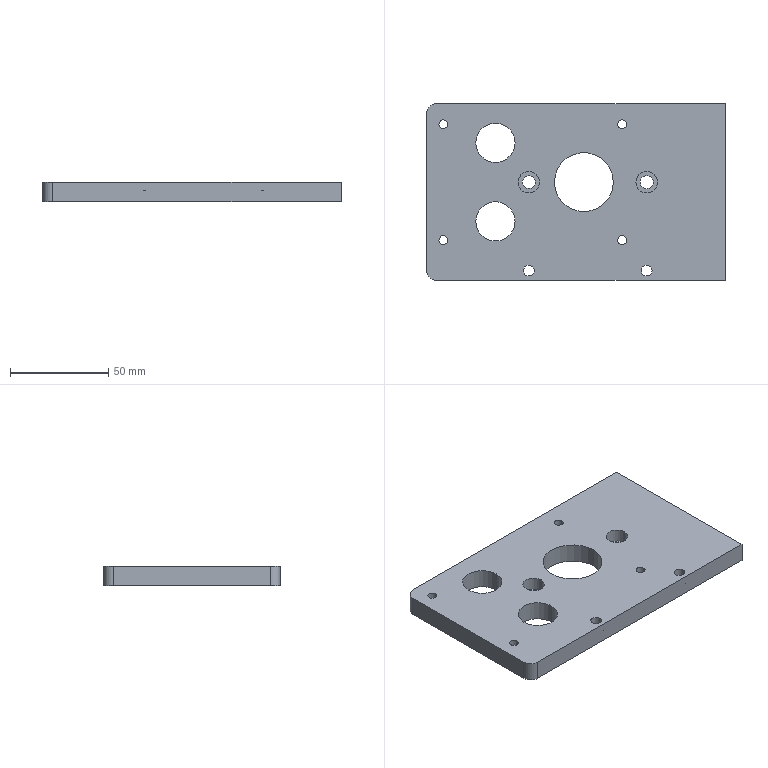Part | SolidWorks | features HoleWzd 4, MoveFace 2, Extrusion 1, Fillet 1, ICE 1 | 1 solid | 62 faces | box 152 x 90 x 10 mm | volume 118972 mm3 | cylinder 44 | plane 14 | cone 4 | commonest cylinder face diameters 4.5 x8 8 x8 4.2 x4 5.5 x4 6.6 x4 9.5 x4